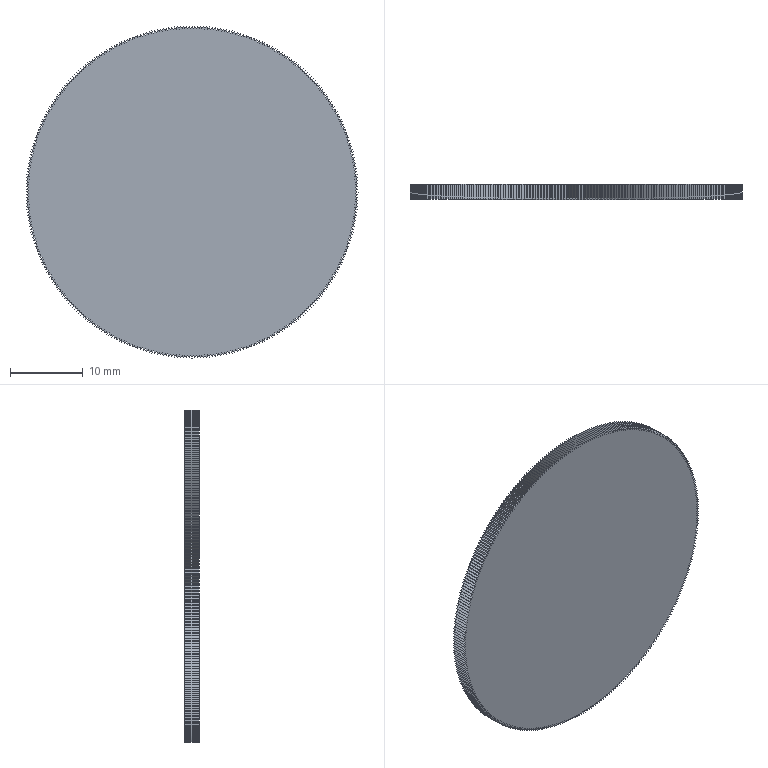Part | SolidWorks | features CirPattern 3, ICE 3, Extrusion 1 | 1 solid | 2740 faces | box 45.5 x 2 x 45.5 mm | volume 3201 mm3 | plane 2740